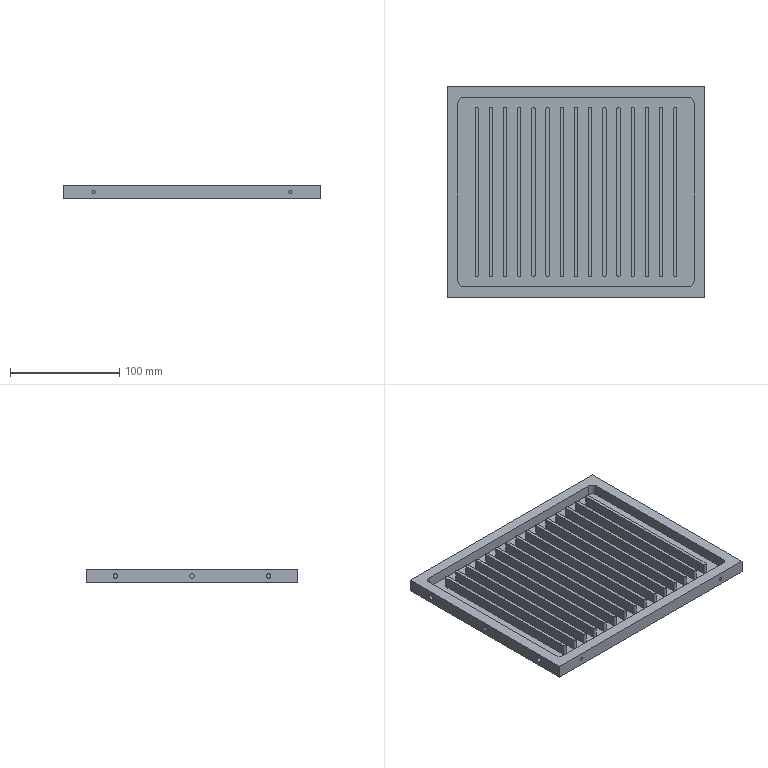Part | SolidWorks | features ICE 4, MirrorPattern 2, Extrusion 1, Fillet 1, LPattern 1 | 1 solid | 120 faces | box 236.3 x 194 x 12 mm | volume 243005 mm3 | plane 66 | cylinder 54 | commonest cylinder face diameters 3 x38 4 x12 10 x4